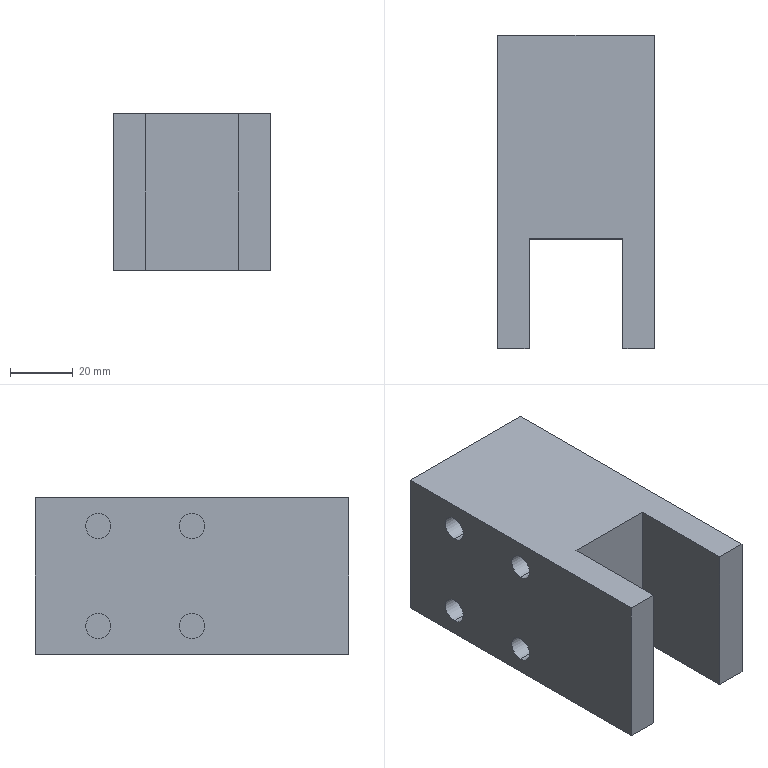Part | SolidWorks | features ICE 4, Extrusion 1 | 1 solid | 37 faces | box 50 x 100 x 50 mm | volume 185436 mm3 | plane 19 | cylinder 18 | commonest cylinder face diameters 8 x16 32 x2
STEP:
#1=CARTESIAN_POINT('',(15.,80.,-20.));
#2=VERTEX_POINT('',#1);
#3=CARTESIAN_POINT('',(15.,80.,-12.));
#4=VERTEX_POINT('',#3);
#5=CARTESIAN_POINT('',(15.,80.,-16.));
#6=DIRECTION('',(-1.,0.,0.));
#7=DIRECTION('',(0.,0.,-1.));
#8=AXIS2_PLACEMENT_3D('',#5,#6,#7);
#9=CIRCLE('',#8,4.);
#10=EDGE_CURVE('',#2,#4,#9,.T.);
#11=ORIENTED_EDGE('',*,*,#10,.T.);
#12=CARTESIAN_POINT('',(25.,80.,-12.));
#13=VERTEX_POINT('',#12);
#14=CARTESIAN_POINT('',(15.,80.,-12.));
#15=DIRECTION('',(1.,0.,0.));
#16=VECTOR('',#15,1000.);
#17=LINE('',#14,#16);
#18=EDGE_CURVE('',#4,#13,#17,.T.);
#19=ORIENTED_EDGE('',*,*,#18,.T.);
#20=CARTESIAN_POINT('',(25.,80.,-20.));
#21=VERTEX_POINT('',#20);
#22=CARTESIAN_POINT('',(25.,80.,-16.));
#23=DIRECTION('',(-1.,0.,0.));
#24=DIRECTION('',(0.,0.,-1.));
#25=AXIS2_PLACEMENT_3D('',#22,#23,#24);
#26=CIRCLE('',#25,4.);
#27=EDGE_CURVE('',#21,#13,#26,.T.);
#28=ORIENTED_EDGE('',*,*,#27,.F.);
#29=CARTESIAN_POINT('',(15.,80.,-20.));
#30=DIRECTION('',(1.,0.,0.));
#31=VECTOR('',#30,1000.);
#32=LINE('',#29,#31);
#33=EDGE_CURVE('',#2,#21,#32,.T.);
#34=ORIENTED_EDGE('',*,*,#33,.F.);
#35=EDGE_LOOP('',(#11,#19,#28,#34));
#36=FACE_OUTER_BOUND('',#35,.T.);
#37=CARTESIAN_POINT('',(15.,80.,-16.));
#38=DIRECTION('',(1.,0.,0.));
#39=DIRECTION('',(0.,0.,-1.));
#40=AXIS2_PLACEMENT_3D('',#37,#38,#39);
#41=CYLINDRICAL_SURFACE('',#40,4.);
#42=ADVANCED_FACE('',(#36),#41,.F.);
#43=CARTESIAN_POINT('',(15.,50.,-20.));
#44=VERTEX_POINT('',#43);
#45=CARTESIAN_POINT('',(15.,50.,-12.));
#46=VERTEX_POINT('',#45);
#47=CARTESIAN_POINT('',(15.,50.,-16.));
#48=DIRECTION('',(-1.,0.,0.));
#49=DIRECTION('',(0.,0.,-1.));
#50=AXIS2_PLACEMENT_3D('',#47,#48,#49);
#51=CIRCLE('',#50,4.);
#52=EDGE_CURVE('',#44,#46,#51,.T.);
#53=ORIENTED_EDGE('',*,*,#52,.T.);
#54=CARTESIAN_POINT('',(25.,50.,-12.));
#55=VERTEX_POINT('',#54);
#56=CARTESIAN_POINT('',(15.,50.,-12.));
#57=DIRECTION('',(1.,0.,0.));
#58=VECTOR('',#57,1000.);
#59=LINE('',#56,#58);
#60=EDGE_CURVE('',#46,#55,#59,.T.);
#61=ORIENTED_EDGE('',*,*,#60,.T.);
#62=CARTESIAN_POINT('',(25.,50.,-20.));
#63=VERTEX_POINT('',#62);
#64=CARTESIAN_POINT('',(25.,50.,-16.));
#65=DIRECTION('',(-1.,0.,0.));
#66=DIRECTION('',(0.,0.,-1.));
#67=AXIS2_PLACEMENT_3D('',#64,#65,#66);
#68=CIRCLE('',#67,4.);
#69=EDGE_CURVE('',#63,#55,#68,.T.);
#70=ORIENTED_EDGE('',*,*,#69,.F.);
#71=CARTESIAN_POINT('',(15.,50.,-20.));
#72=DIRECTION('',(1.,0.,0.));
#73=VECTOR('',#72,1000.);
#74=LINE('',#71,#73);
#75=EDGE_CURVE('',#44,#63,#74,.T.);
#76=ORIENTED_EDGE('',*,*,#75,.F.);
#77=EDGE_LOOP('',(#53,#61,#70,#76));
#78=FACE_OUTER_BOUND('',#77,.T.);
#79=CARTESIAN_POINT('',(15.,50.,-16.));
#80=DIRECTION('',(1.,0.,0.));
#81=DIRECTION('',(0.,0.,-1.));
#82=AXIS2_PLACEMENT_3D('',#79,#80,#81);
#83=CYLINDRICAL_SURFACE('',#82,4.);
#84=ADVANCED_FACE('',(#78),#83,.F.);
#85=CARTESIAN_POINT('',(15.,50.,20.));
#86=VERTEX_POINT('',#85);
#87=CARTESIAN_POINT('',(15.,50.,12.));
#88=VERTEX_POINT('',#87);
#89=CARTESIAN_POINT('',(15.,50.,16.));
#90=DIRECTION('',(1.,0.,0.));
#91=DIRECTION('',(0.,0.,-1.));
#92=AXIS2_PLACEMENT_3D('',#89,#90,#91);
#93=CIRCLE('',#92,4.);
#94=EDGE_CURVE('',#86,#88,#93,.T.);
#95=ORIENTED_EDGE('',*,*,#94,.F.);
#96=CARTESIAN_POINT('',(25.,50.,20.));
#97=VERTEX_POINT('',#96);
#98=CARTESIAN_POINT('',(15.,50.,20.));
#99=DIRECTION('',(1.,0.,0.));
#100=VECTOR('',#99,1000.);
#101=LINE('',#98,#100);
#102=EDGE_CURVE('',#86,#97,#101,.T.);
#103=ORIENTED_EDGE('',*,*,#102,.T.);
#104=CARTESIAN_POINT('',(25.,50.,12.));
#105=VERTEX_POINT('',#104);
#106=CARTESIAN_POINT('',(25.,50.,16.));
#107=DIRECTION('',(1.,0.,0.));
#108=DIRECTION('',(0.,0.,-1.));
#109=AXIS2_PLACEMENT_3D('',#106,#107,#108);
#110=CIRCLE('',#109,4.);
#111=EDGE_CURVE('',#97,#105,#110,.T.);
#112=ORIENTED_EDGE('',*,*,#111,.T.);
#113=CARTESIAN_POINT('',(15.,50.,12.));
#114=DIRECTION('',(1.,0.,0.));
#115=VECTOR('',#114,1000.);
#116=LINE('',#113,#115);
#117=EDGE_CURVE('',#88,#105,#116,.T.);
#118=ORIENTED_EDGE('',*,*,#117,.F.);
#119=EDGE_LOOP('',(#95,#103,#112,#118));
#120=FACE_OUTER_BOUND('',#119,.T.);
#121=CARTESIAN_POINT('',(15.,50.,16.));
#122=DIRECTION('',(1.,0.,0.));
#123=DIRECTION('',(0.,0.,-1.));
#124=AXIS2_PLACEMENT_3D('',#121,#122,#123);
#125=CYLINDRICAL_SURFACE('',#124,4.);
#126=ADVANCED_FACE('',(#120),#125,.F.);
#127=CARTESIAN_POINT('',(15.,80.,20.));
#128=VERTEX_POINT('',#127);
#129=CARTESIAN_POINT('',(15.,80.,12.));
#130=VERTEX_POINT('',#129);
#131=CARTESIAN_POINT('',(15.,80.,16.));
#132=DIRECTION('',(1.,0.,0.));
#133=DIRECTION('',(0.,0.,-1.));
#134=AXIS2_PLACEMENT_3D('',#131,#132,#133);
#135=CIRCLE('',#134,4.);
#136=EDGE_CURVE('',#128,#130,#135,.T.);
#137=ORIENTED_EDGE('',*,*,#136,.F.);
#138=CARTESIAN_POINT('',(25.,80.,20.));
#139=VERTEX_POINT('',#138);
#140=CARTESIAN_POINT('',(15.,80.,20.));
#141=DIRECTION('',(1.,0.,0.));
#142=VECTOR('',#141,1000.);
#143=LINE('',#140,#142);
#144=EDGE_CURVE('',#128,#139,#143,.T.);
#145=ORIENTED_EDGE('',*,*,#144,.T.);
#146=CARTESIAN_POINT('',(25.,80.,12.));
#147=VERTEX_POINT('',#146);
#148=CARTESIAN_POINT('',(25.,80.,16.));
#149=DIRECTION('',(1.,0.,0.));
#150=DIRECTION('',(0.,0.,-1.));
#151=AXIS2_PLACEMENT_3D('',#148,#149,#150);
#152=CIRCLE('',#151,4.);
#153=EDGE_CURVE('',#139,#147,#152,.T.);
#154=ORIENTED_EDGE('',*,*,#153,.T.);
#155=CARTESIAN_POINT('',(15.,80.,12.));
#156=DIRECTION('',(1.,0.,0.));
#157=VECTOR('',#156,1000.);
#158=LINE('',#155,#157);
#159=EDGE_CURVE('',#130,#147,#158,.T.);
#160=ORIENTED_EDGE('',*,*,#159,.F.);
#161=EDGE_LOOP('',(#137,#145,#154,#160));
#162=FACE_OUTER_BOUND('',#161,.T.);
#163=CARTESIAN_POINT('',(15.,80.,16.));
#164=DIRECTION('',(1.,0.,0.));
#165=DIRECTION('',(0.,0.,-1.));
#166=AXIS2_PLACEMENT_3D('',#163,#164,#165);
#167=CYLINDRICAL_SURFACE('',#166,4.);
#168=ADVANCED_FACE('',(#162),#167,.F.);
#169=CARTESIAN_POINT('',(-15.,50.,-20.));
#170=VERTEX_POINT('',#169);
#171=CARTESIAN_POINT('',(-15.,50.,-12.));
#172=VERTEX_POINT('',#171);
#173=CARTESIAN_POINT('',(-15.,50.,-16.));
#174=DIRECTION('',(-1.,0.,0.));
#175=DIRECTION('',(0.,0.,1.));
#176=AXIS2_PLACEMENT_3D('',#173,#174,#175);
#177=CIRCLE('',#176,4.);
#178=EDGE_CURVE('',#170,#172,#177,.T.);
#179=ORIENTED_EDGE('',*,*,#178,.F.);
#180=CARTESIAN_POINT('',(-25.,50.,-20.));
#181=VERTEX_POINT('',#180);
#182=CARTESIAN_POINT('',(-15.,50.,-20.));
#183=DIRECTION('',(-1.,0.,0.));
#184=VECTOR('',#183,1000.);
#185=LINE('',#182,#184);
#186=EDGE_CURVE('',#170,#181,#185,.T.);
#187=ORIENTED_EDGE('',*,*,#186,.T.);
#188=CARTESIAN_POINT('',(-25.,50.,-12.));
#189=VERTEX_POINT('',#188);
#190=CARTESIAN_POINT('',(-25.,50.,-16.));
#191=DIRECTION('',(-1.,0.,0.));
#192=DIRECTION('',(0.,0.,1.));
#193=AXIS2_PLACEMENT_3D('',#190,#191,#192);
#194=CIRCLE('',#193,4.);
#195=EDGE_CURVE('',#181,#189,#194,.T.);
#196=ORIENTED_EDGE('',*,*,#195,.T.);
#197=CARTESIAN_POINT('',(-15.,50.,-12.));
#198=DIRECTION('',(-1.,0.,0.));
#199=VECTOR('',#198,1000.);
#200=LINE('',#197,#199);
#201=EDGE_CURVE('',#172,#189,#200,.T.);
#202=ORIENTED_EDGE('',*,*,#201,.F.);
#203=EDGE_LOOP('',(#179,#187,#196,#202));
#204=FACE_OUTER_BOUND('',#203,.T.);
#205=CARTESIAN_POINT('',(-15.,50.,-16.));
#206=DIRECTION('',(-1.,0.,0.));
#207=DIRECTION('',(0.,0.,1.));
#208=AXIS2_PLACEMENT_3D('',#205,#206,#207);
#209=CYLINDRICAL_SURFACE('',#208,4.);
#210=ADVANCED_FACE('',(#204),#209,.F.);
#211=CARTESIAN_POINT('',(-15.,50.,20.));
#212=VERTEX_POINT('',#211);
#213=CARTESIAN_POINT('',(-15.,50.,12.));
#214=VERTEX_POINT('',#213);
#215=CARTESIAN_POINT('',(-15.,50.,16.));
#216=DIRECTION('',(1.,0.,0.));
#217=DIRECTION('',(0.,0.,1.));
#218=AXIS2_PLACEMENT_3D('',#215,#216,#217);
#219=CIRCLE('',#218,4.);
#220=EDGE_CURVE('',#212,#214,#219,.T.);
#221=ORIENTED_EDGE('',*,*,#220,.T.);
#222=CARTESIAN_POINT('',(-25.,50.,12.));
#223=VERTEX_POINT('',#222);
#224=CARTESIAN_POINT('',(-15.,50.,12.));
#225=DIRECTION('',(-1.,0.,0.));
#226=VECTOR('',#225,1000.);
#227=LINE('',#224,#226);
#228=EDGE_CURVE('',#214,#223,#227,.T.);
#229=ORIENTED_EDGE('',*,*,#228,.T.);
#230=CARTESIAN_POINT('',(-25.,50.,20.));
#231=VERTEX_POINT('',#230);
#232=CARTESIAN_POINT('',(-25.,50.,16.));
#233=DIRECTION('',(1.,0.,0.));
#234=DIRECTION('',(0.,0.,1.));
#235=AXIS2_PLACEMENT_3D('',#232,#233,#234);
#236=CIRCLE('',#235,4.);
#237=EDGE_CURVE('',#231,#223,#236,.T.);
#238=ORIENTED_EDGE('',*,*,#237,.F.);
#239=CARTESIAN_POINT('',(-15.,50.,20.));
#240=DIRECTION('',(-1.,0.,0.));
#241=VECTOR('',#240,1000.);
#242=LINE('',#239,#241);
#243=EDGE_CURVE('',#212,#231,#242,.T.);
#244=ORIENTED_EDGE('',*,*,#243,.F.);
#245=EDGE_LOOP('',(#221,#229,#238,#244));
#246=FACE_OUTER_BOUND('',#245,.T.);
#247=CARTESIAN_POINT('',(-15.,50.,16.));
#248=DIRECTION('',(-1.,0.,0.));
#249=DIRECTION('',(0.,0.,1.));
#250=AXIS2_PLACEMENT_3D('',#247,#248,#249);
#251=CYLINDRICAL_SURFACE('',#250,4.);
#252=ADVANCED_FACE('',(#246),#251,.F.);
#253=CARTESIAN_POINT('',(-15.,80.,20.));
#254=VERTEX_POINT('',#253);
#255=CARTESIAN_POINT('',(-15.,80.,12.));
#256=VERTEX_POINT('',#255);
#257=CARTESIAN_POINT('',(-15.,80.,16.));
#258=DIRECTION('',(1.,0.,0.));
#259=DIRECTION('',(0.,0.,1.));
#260=AXIS2_PLACEMENT_3D('',#257,#258,#259);
#261=CIRCLE('',#260,4.);
#262=EDGE_CURVE('',#254,#256,#261,.T.);
#263=ORIENTED_EDGE('',*,*,#262,.T.);
#264=CARTESIAN_POINT('',(-25.,80.,12.));
#265=VERTEX_POINT('',#264);
#266=CARTESIAN_POINT('',(-15.,80.,12.));
#267=DIRECTION('',(-1.,0.,0.));
#268=VECTOR('',#267,1000.);
#269=LINE('',#266,#268);
#270=EDGE_CURVE('',#256,#265,#269,.T.);
#271=ORIENTED_EDGE('',*,*,#270,.T.);
#272=CARTESIAN_POINT('',(-25.,80.,20.));
#273=VERTEX_POINT('',#272);
#274=CARTESIAN_POINT('',(-25.,80.,16.));
#275=DIRECTION('',(1.,0.,0.));
#276=DIRECTION('',(0.,0.,1.));
#277=AXIS2_PLACEMENT_3D('',#274,#275,#276);
#278=CIRCLE('',#277,4.);
#279=EDGE_CURVE('',#273,#265,#278,.T.);
#280=ORIENTED_EDGE('',*,*,#279,.F.);
#281=CARTESIAN_POINT('',(-15.,80.,20.));
#282=DIRECTION('',(-1.,0.,0.));
#283=VECTOR('',#282,1000.);
#284=LINE('',#281,#283);
#285=EDGE_CURVE('',#254,#273,#284,.T.);
#286=ORIENTED_EDGE('',*,*,#285,.F.);
#287=EDGE_LOOP('',(#263,#271,#280,#286));
#288=FACE_OUTER_BOUND('',#287,.T.);
#289=CARTESIAN_POINT('',(-15.,80.,16.));
#290=DIRECTION('',(-1.,0.,0.));
#291=DIRECTION('',(0.,0.,1.));
#292=AXIS2_PLACEMENT_3D('',#289,#290,#291);
#293=CYLINDRICAL_SURFACE('',#292,4.);
#294=ADVANCED_FACE('',(#288),#293,.F.);
#295=CARTESIAN_POINT('',(-15.,80.,-20.));
#296=VERTEX_POINT('',#295);
#297=CARTESIAN_POINT('',(-15.,80.,-12.));
#298=VERTEX_POINT('',#297);
#299=CARTESIAN_POINT('',(-15.,80.,-16.));
#300=DIRECTION('',(-1.,0.,0.));
#301=DIRECTION('',(0.,0.,1.));
#302=AXIS2_PLACEMENT_3D('',#299,#300,#301);
#303=CIRCLE('',#302,4.);
#304=EDGE_CURVE('',#296,#298,#303,.T.);
#305=ORIENTED_EDGE('',*,*,#304,.F.);
#306=CARTESIAN_POINT('',(-25.,80.,-20.));
#307=VERTEX_POINT('',#306);
#308=CARTESIAN_POINT('',(-15.,80.,-20.));
#309=DIRECTION('',(-1.,0.,0.));
#310=VECTOR('',#309,1000.);
#311=LINE('',#308,#310);
#312=EDGE_CURVE('',#296,#307,#311,.T.);
#313=ORIENTED_EDGE('',*,*,#312,.T.);
#314=CARTESIAN_POINT('',(-25.,80.,-12.));
#315=VERTEX_POINT('',#314);
#316=CARTESIAN_POINT('',(-25.,80.,-16.));
#317=DIRECTION('',(-1.,0.,0.));
#318=DIRECTION('',(0.,0.,1.));
#319=AXIS2_PLACEMENT_3D('',#316,#317,#318);
#320=CIRCLE('',#319,4.);
#321=EDGE_CURVE('',#307,#315,#320,.T.);
#322=ORIENTED_EDGE('',*,*,#321,.T.);
#323=CARTESIAN_POINT('',(-15.,80.,-12.));
#324=DIRECTION('',(-1.,0.,0.));
#325=VECTOR('',#324,1000.);
#326=LINE('',#323,#325);
#327=EDGE_CURVE('',#298,#315,#326,.T.);
#328=ORIENTED_EDGE('',*,*,#327,.F.);
#329=EDGE_LOOP('',(#305,#313,#322,#328));
#330=FACE_OUTER_BOUND('',#329,.T.);
#331=CARTESIAN_POINT('',(-15.,80.,-16.));
#332=DIRECTION('',(-1.,0.,0.));
#333=DIRECTION('',(0.,0.,1.));
#334=AXIS2_PLACEMENT_3D('',#331,#332,#333);
#335=CYLINDRICAL_SURFACE('',#334,4.);
#336=ADVANCED_FACE('',(#330),#335,.F.);
#337=CARTESIAN_POINT('',(0.,90.,-16.));
#338=VERTEX_POINT('',#337);
#339=CARTESIAN_POINT('',(0.,90.,16.));
#340=VERTEX_POINT('',#339);
#341=CARTESIAN_POINT('',(0.,90.,0.));
#342=DIRECTION('',(0.,1.,0.));
#343=DIRECTION('',(0.,0.,1.));
#344=AXIS2_PLACEMENT_3D('',#341,#342,#343);
#345=CIRCLE('',#344,16.);
#346=EDGE_CURVE('',#338,#340,#345,.T.);
#347=ORIENTED_EDGE('',*,*,#346,.F.);
#348=CARTESIAN_POINT('',(0.,100.,-16.));
#349=VERTEX_POINT('',#348);
#350=CARTESIAN_POINT('',(0.,90.,-16.));
#351=DIRECTION('',(0.,1.,0.));
#352=VECTOR('',#351,1000.);
#353=LINE('',#350,#352);
#354=EDGE_CURVE('',#338,#349,#353,.T.);
#355=ORIENTED_EDGE('',*,*,#354,.T.);
#356=CARTESIAN_POINT('',(0.,100.,16.));
#357=VERTEX_POINT('',#356);
#358=CARTESIAN_POINT('',(0.,100.,0.));
#359=DIRECTION('',(0.,1.,0.));
#360=DIRECTION('',(0.,0.,1.));
#361=AXIS2_PLACEMENT_3D('',#358,#359,#360);
#362=CIRCLE('',#361,16.);
#363=EDGE_CURVE('',#349,#357,#362,.T.);
#364=ORIENTED_EDGE('',*,*,#363,.T.);
#365=CARTESIAN_POINT('',(0.,90.,16.));
#366=DIRECTION('',(0.,1.,0.));
#367=VECTOR('',#366,1000.);
#368=LINE('',#365,#367);
#369=EDGE_CURVE('',#340,#357,#368,.T.);
#370=ORIENTED_EDGE('',*,*,#369,.F.);
#371=EDGE_LOOP('',(#347,#355,#364,#370));
#372=FACE_OUTER_BOUND('',#371,.T.);
#373=CARTESIAN_POINT('',(0.,90.,0.));
#374=DIRECTION('',(0.,1.,0.));
#375=DIRECTION('',(0.,0.,1.));
#376=AXIS2_PLACEMENT_3D('',#373,#374,#375);
#377=CYLINDRICAL_SURFACE('',#376,16.);
#378=ADVANCED_FACE('',(#372),#377,.F.);
#379=CARTESIAN_POINT('',(25.,50.,16.));
#380=DIRECTION('',(1.,0.,0.));
#381=DIRECTION('',(0.,0.,-1.));
#382=AXIS2_PLACEMENT_3D('',#379,#380,#381);
#383=CIRCLE('',#382,4.);
#384=EDGE_CURVE('',#105,#97,#383,.T.);
#385=ORIENTED_EDGE('',*,*,#384,.F.);
#386=ORIENTED_EDGE('',*,*,#111,.F.);
#387=EDGE_LOOP('',(#385,#386));
#388=FACE_BOUND('',#387,.T.);
#389=CARTESIAN_POINT('',(25.,80.,16.));
#390=DIRECTION('',(1.,0.,0.));
#391=DIRECTION('',(0.,0.,-1.));
#392=AXIS2_PLACEMENT_3D('',#389,#390,#391);
#393=CIRCLE('',#392,4.);
#394=EDGE_CURVE('',#147,#139,#393,.T.);
#395=ORIENTED_EDGE('',*,*,#394,.F.);
#396=ORIENTED_EDGE('',*,*,#153,.F.);
#397=EDGE_LOOP('',(#395,#396));
#398=FACE_BOUND('',#397,.T.);
#399=CARTESIAN_POINT('',(25.,0.,25.));
#400=VERTEX_POINT('',#399);
#401=CARTESIAN_POINT('',(25.,0.,-25.));
#402=VERTEX_POINT('',#401);
#403=CARTESIAN_POINT('',(25.,0.,-25.));
#404=DIRECTION('',(0.,0.,-1.));
#405=VECTOR('',#404,1000.);
#406=LINE('',#403,#405);
#407=EDGE_CURVE('',#400,#402,#406,.T.);
#408=ORIENTED_EDGE('',*,*,#407,.T.);
#409=CARTESIAN_POINT('',(25.,100.,-25.));
#410=VERTEX_POINT('',#409);
#411=CARTESIAN_POINT('',(25.,100.,-25.));
#412=DIRECTION('',(0.,-1.,0.));
#413=VECTOR('',#412,1000.);
#414=LINE('',#411,#413);
#415=EDGE_CURVE('',#410,#402,#414,.T.);
#416=ORIENTED_EDGE('',*,*,#415,.F.);
#417=CARTESIAN_POINT('',(25.,100.,25.));
#418=VERTEX_POINT('',#417);
#419=CARTESIAN_POINT('',(25.,100.,-25.));
#420=DIRECTION('',(0.,0.,-1.));
#421=VECTOR('',#420,1000.);
#422=LINE('',#419,#421);
#423=EDGE_CURVE('',#418,#410,#422,.T.);
#424=ORIENTED_EDGE('',*,*,#423,.F.);
#425=CARTESIAN_POINT('',(25.,100.,25.));
#426=DIRECTION('',(0.,-1.,0.));
#427=VECTOR('',#426,1000.);
#428=LINE('',#425,#427);
#429=EDGE_CURVE('',#418,#400,#428,.T.);
#430=ORIENTED_EDGE('',*,*,#429,.T.);
#431=EDGE_LOOP('',(#408,#416,#424,#430));
#432=FACE_OUTER_BOUND('',#431,.T.);
#433=ORIENTED_EDGE('',*,*,#69,.T.);
#434=CARTESIAN_POINT('',(25.,50.,-16.));
#435=DIRECTION('',(-1.,0.,0.));
#436=DIRECTION('',(0.,0.,-1.));
#437=AXIS2_PLACEMENT_3D('',#434,#435,#436);
#438=CIRCLE('',#437,4.);
#439=EDGE_CURVE('',#55,#63,#438,.T.);
#440=ORIENTED_EDGE('',*,*,#439,.T.);
#441=EDGE_LOOP('',(#433,#440));
#442=FACE_BOUND('',#441,.T.);
#443=ORIENTED_EDGE('',*,*,#27,.T.);
#444=CARTESIAN_POINT('',(25.,80.,-16.));
#445=DIRECTION('',(-1.,0.,0.));
#446=DIRECTION('',(0.,0.,-1.));
#447=AXIS2_PLACEMENT_3D('',#444,#445,#446);
#448=CIRCLE('',#447,4.);
#449=EDGE_CURVE('',#13,#21,#448,.T.);
#450=ORIENTED_EDGE('',*,*,#449,.T.);
#451=EDGE_LOOP('',(#443,#450));
#452=FACE_BOUND('',#451,.T.);
#453=CARTESIAN_POINT('',(25.,100.,-25.));
#454=DIRECTION('',(-1.,0.,0.));
#455=DIRECTION('',(0.,0.,1.));
#456=AXIS2_PLACEMENT_3D('',#453,#454,#455);
#457=PLANE('',#456);
#458=ADVANCED_FACE('',(#388,#398,#432,#442,#452),#457,.F.);
#459=CARTESIAN_POINT('',(-25.,50.,-16.));
#460=DIRECTION('',(-1.,0.,0.));
#461=DIRECTION('',(0.,0.,1.));
#462=AXIS2_PLACEMENT_3D('',#459,#460,#461);
#463=CIRCLE('',#462,4.);
#464=EDGE_CURVE('',#189,#181,#463,.T.);
#465=ORIENTED_EDGE('',*,*,#464,.F.);
#466=ORIENTED_EDGE('',*,*,#195,.F.);
#467=EDGE_LOOP('',(#465,#466));
#468=FACE_BOUND('',#467,.T.);
#469=CARTESIAN_POINT('',(-25.,80.,-16.));
#470=DIRECTION('',(-1.,0.,0.));
#471=DIRECTION('',(0.,0.,1.));
#472=AXIS2_PLACEMENT_3D('',#469,#470,#471);
#473=CIRCLE('',#472,4.);
#474=EDGE_CURVE('',#315,#307,#473,.T.);
#475=ORIENTED_EDGE('',*,*,#474,.F.);
#476=ORIENTED_EDGE('',*,*,#321,.F.);
#477=EDGE_LOOP('',(#475,#476));
#478=FACE_BOUND('',#477,.T.);
#479=CARTESIAN_POINT('',(-25.,0.,-25.));
#480=VERTEX_POINT('',#479);
#481=CARTESIAN_POINT('',(-25.,0.,25.));
#482=VERTEX_POINT('',#481);
#483=CARTESIAN_POINT('',(-25.,0.,-25.));
#484=DIRECTION('',(0.,0.,1.));
#485=VECTOR('',#484,1000.);
#486=LINE('',#483,#485);
#487=EDGE_CURVE('',#480,#482,#486,.T.);
#488=ORIENTED_EDGE('',*,*,#487,.T.);
#489=CARTESIAN_POINT('',(-25.,100.,25.));
#490=VERTEX_POINT('',#489);
#491=CARTESIAN_POINT('',(-25.,100.,25.));
#492=DIRECTION('',(0.,-1.,0.));
#493=VECTOR('',#492,1000.);
#494=LINE('',#491,#493);
#495=EDGE_CURVE('',#490,#482,#494,.T.);
#496=ORIENTED_EDGE('',*,*,#495,.F.);
#497=CARTESIAN_POINT('',(-25.,100.,-25.));
#498=VERTEX_POINT('',#497);
#499=CARTESIAN_POINT('',(-25.,100.,-25.));
#500=DIRECTION('',(0.,0.,1.));
#501=VECTOR('',#500,1000.);
#502=LINE('',#499,#501);
#503=EDGE_CURVE('',#498,#490,#502,.T.);
#504=ORIENTED_EDGE('',*,*,#503,.F.);
#505=CARTESIAN_POINT('',(-25.,100.,-25.));
#506=DIRECTION('',(0.,-1.,0.));
#507=VECTOR('',#506,1000.);
#508=LINE('',#505,#507);
#509=EDGE_CURVE('',#498,#480,#508,.T.);
#510=ORIENTED_EDGE('',*,*,#509,.T.);
#511=EDGE_LOOP('',(#488,#496,#504,#510));
#512=FACE_OUTER_BOUND('',#511,.T.);
#513=ORIENTED_EDGE('',*,*,#279,.T.);
#514=CARTESIAN_POINT('',(-25.,80.,16.));
#515=DIRECTION('',(1.,0.,0.));
#516=DIRECTION('',(0.,0.,1.));
#517=AXIS2_PLACEMENT_3D('',#514,#515,#516);
#518=CIRCLE('',#517,4.);
#519=EDGE_CURVE('',#265,#273,#518,.T.);
#520=ORIENTED_EDGE('',*,*,#519,.T.);
#521=EDGE_LOOP('',(#513,#520));
#522=FACE_BOUND('',#521,.T.);
#523=ORIENTED_EDGE('',*,*,#237,.T.);
#524=CARTESIAN_POINT('',(-25.,50.,16.));
#525=DIRECTION('',(1.,0.,0.));
#526=DIRECTION('',(0.,0.,1.));
#527=AXIS2_PLACEMENT_3D('',#524,#525,#526);
#528=CIRCLE('',#527,4.);
#529=EDGE_CURVE('',#223,#231,#528,.T.);
#530=ORIENTED_EDGE('',*,*,#529,.T.);
#531=EDGE_LOOP('',(#523,#530));
#532=FACE_BOUND('',#531,.T.);
#533=CARTESIAN_POINT('',(-25.,100.,-25.));
#534=DIRECTION('',(1.,0.,0.));
#535=DIRECTION('',(0.,0.,-1.));
#536=AXIS2_PLACEMENT_3D('',#533,#534,#535);
#537=PLANE('',#536);
#538=ADVANCED_FACE('',(#468,#478,#512,#522,#532),#537,.F.);
#539=CARTESIAN_POINT('',(15.,0.,25.));
#540=VERTEX_POINT('',#539);
#541=CARTESIAN_POINT('',(-25.,0.,25.));
#542=DIRECTION('',(1.,0.,0.));
#543=VECTOR('',#542,1000.);
#544=LINE('',#541,#543);
#545=EDGE_CURVE('',#540,#400,#544,.T.);
#546=ORIENTED_EDGE('',*,*,#545,.F.);
#547=CARTESIAN_POINT('',(15.,0.,-25.));
#548=VERTEX_POINT('',#547);
#549=CARTESIAN_POINT('',(15.,0.,25.));
#550=DIRECTION('',(0.,0.,1.));
#551=VECTOR('',#550,1000.);
#552=LINE('',#549,#551);
#553=EDGE_CURVE('',#548,#540,#552,.T.);
#554=ORIENTED_EDGE('',*,*,#553,.F.);
#555=CARTESIAN_POINT('',(-25.,0.,-25.));
#556=DIRECTION('',(-1.,0.,0.));
#557=VECTOR('',#556,1000.);
#558=LINE('',#555,#557);
#559=EDGE_CURVE('',#402,#548,#558,.T.);
#560=ORIENTED_EDGE('',*,*,#559,.F.);
#561=ORIENTED_EDGE('',*,*,#407,.F.);
#562=EDGE_LOOP('',(#546,#554,#560,#561));
#563=FACE_OUTER_BOUND('',#562,.T.);
#564=CARTESIAN_POINT('',(0.,0.,0.));
#565=DIRECTION('',(0.,1.,0.));
#566=DIRECTION('',(0.,0.,1.));
#567=AXIS2_PLACEMENT_3D('',#564,#565,#566);
#568=PLANE('',#567);
#569=ADVANCED_FACE('',(#563),#568,.F.);
#570=ORIENTED_EDGE('',*,*,#559,.T.);
#571=CARTESIAN_POINT('',(15.,35.,-25.));
#572=VERTEX_POINT('',#571);
#573=CARTESIAN_POINT('',(15.,35.,-25.));
#574=DIRECTION('',(0.,-1.,0.));
#575=VECTOR('',#574,1000.);
#576=LINE('',#573,#575);
#577=EDGE_CURVE('',#572,#548,#576,.T.);
#578=ORIENTED_EDGE('',*,*,#577,.F.);
#579=CARTESIAN_POINT('',(-15.,35.,-25.));
#580=VERTEX_POINT('',#579);
#581=CARTESIAN_POINT('',(-15.,35.,-25.));
#582=DIRECTION('',(1.,0.,0.));
#583=VECTOR('',#582,1000.);
#584=LINE('',#581,#583);
#585=EDGE_CURVE('',#580,#572,#584,.T.);
#586=ORIENTED_EDGE('',*,*,#585,.F.);
#587=CARTESIAN_POINT('',(-15.,0.,-25.));
#588=VERTEX_POINT('',#587);
#589=CARTESIAN_POINT('',(-15.,35.,-25.));
#590=DIRECTION('',(0.,-1.,0.));
#591=VECTOR('',#590,1000.);
#592=LINE('',#589,#591);
#593=EDGE_CURVE('',#580,#588,#592,.T.);
#594=ORIENTED_EDGE('',*,*,#593,.T.);
#595=CARTESIAN_POINT('',(-25.,0.,-25.));
#596=DIRECTION('',(-1.,0.,0.));
#597=VECTOR('',#596,1000.);
#598=LINE('',#595,#597);
#599=EDGE_CURVE('',#588,#480,#598,.T.);
#600=ORIENTED_EDGE('',*,*,#599,.T.);
#601=ORIENTED_EDGE('',*,*,#509,.F.);
#602=CARTESIAN_POINT('',(-25.,100.,-25.));
#603=DIRECTION('',(-1.,0.,0.));
#604=VECTOR('',#603,1000.);
#605=LINE('',#602,#604);
#606=EDGE_CURVE('',#410,#498,#605,.T.);
#607=ORIENTED_EDGE('',*,*,#606,.F.);
#608=ORIENTED_EDGE('',*,*,#415,.T.);
#609=EDGE_LOOP('',(#570,#578,#586,#594,#600,#601,#607,#608));
#610=FACE_OUTER_BOUND('',#609,.T.);
#611=CARTESIAN_POINT('',(-25.,100.,-25.));
#612=DIRECTION('',(0.,0.,1.));
#613=DIRECTION('',(1.,0.,0.));
#614=AXIS2_PLACEMENT_3D('',#611,#612,#613);
#615=PLANE('',#614);
#616=ADVANCED_FACE('',(#610),#615,.F.);
#617=CARTESIAN_POINT('',(15.,35.,25.));
#618=VERTEX_POINT('',#617);
#619=CARTESIAN_POINT('',(-15.,35.,25.));
#620=VERTEX_POINT('',#619);
#621=CARTESIAN_POINT('',(-15.,35.,25.));
#622=DIRECTION('',(-1.,0.,0.));
#623=VECTOR('',#622,1000.);
#624=LINE('',#621,#623);
#625=EDGE_CURVE('',#618,#620,#624,.T.);
#626=ORIENTED_EDGE('',*,*,#625,.F.);
#627=CARTESIAN_POINT('',(15.,35.,25.));
#628=DIRECTION('',(0.,-1.,0.));
#629=VECTOR('',#628,1000.);
#630=LINE('',#627,#629);
#631=EDGE_CURVE('',#618,#540,#630,.T.);
#632=ORIENTED_EDGE('',*,*,#631,.T.);
#633=ORIENTED_EDGE('',*,*,#545,.T.);
#634=ORIENTED_EDGE('',*,*,#429,.F.);
#635=CARTESIAN_POINT('',(-25.,100.,25.));
#636=DIRECTION('',(1.,0.,0.));
#637=VECTOR('',#636,1000.);
#638=LINE('',#635,#637);
#639=EDGE_CURVE('',#490,#418,#638,.T.);
#640=ORIENTED_EDGE('',*,*,#639,.F.);
#641=ORIENTED_EDGE('',*,*,#495,.T.);
#642=CARTESIAN_POINT('',(-15.,0.,25.));
#643=VERTEX_POINT('',#642);
#644=CARTESIAN_POINT('',(-25.,0.,25.));
#645=DIRECTION('',(1.,0.,0.));
#646=VECTOR('',#645,1000.);
#647=LINE('',#644,#646);
#648=EDGE_CURVE('',#482,#643,#647,.T.);
#649=ORIENTED_EDGE('',*,*,#648,.T.);
#650=CARTESIAN_POINT('',(-15.,35.,25.));
#651=DIRECTION('',(0.,-1.,0.));
#652=VECTOR('',#651,1000.);
#653=LINE('',#650,#652);
#654=EDGE_CURVE('',#620,#643,#653,.T.);
#655=ORIENTED_EDGE('',*,*,#654,.F.);
#656=EDGE_LOOP('',(#626,#632,#633,#634,#640,#641,#649,#655));
#657=FACE_OUTER_BOUND('',#656,.T.);
#658=CARTESIAN_POINT('',(-25.,100.,25.));
#659=DIRECTION('',(0.,0.,-1.));
#660=DIRECTION('',(-1.,0.,0.));
#661=AXIS2_PLACEMENT_3D('',#658,#659,#660);
#662=PLANE('',#661);
#663=ADVANCED_FACE('',(#657),#662,.F.);
#664=CARTESIAN_POINT('',(0.,100.,0.));
#665=DIRECTION('',(0.,1.,0.));
#666=DIRECTION('',(0.,0.,1.));
#667=AXIS2_PLACEMENT_3D('',#664,#665,#666);
#668=CIRCLE('',#667,16.);
#669=EDGE_CURVE('',#357,#349,#668,.T.);
#670=ORIENTED_EDGE('',*,*,#669,.F.);
#671=ORIENTED_EDGE('',*,*,#363,.F.);
#672=EDGE_LOOP('',(#670,#671));
#673=FACE_BOUND('',#672,.T.);
#674=ORIENTED_EDGE('',*,*,#423,.T.);
#675=ORIENTED_EDGE('',*,*,#606,.T.);
#676=ORIENTED_EDGE('',*,*,#503,.T.);
#677=ORIENTED_EDGE('',*,*,#639,.T.);
#678=EDGE_LOOP('',(#674,#675,#676,#677));
#679=FACE_OUTER_BOUND('',#678,.T.);
#680=CARTESIAN_POINT('',(0.,100.,0.));
#681=DIRECTION('',(0.,1.,0.));
#682=DIRECTION('',(0.,0.,1.));
#683=AXIS2_PLACEMENT_3D('',#680,#681,#682);
#684=PLANE('',#683);
#685=ADVANCED_FACE('',(#673,#679),#684,.T.);
#686=ORIENTED_EDGE('',*,*,#599,.F.);
#687=CARTESIAN_POINT('',(-15.,0.,25.));
#688=DIRECTION('',(0.,0.,-1.));
#689=VECTOR('',#688,1000.);
#690=LINE('',#687,#689);
#691=EDGE_CURVE('',#643,#588,#690,.T.);
#692=ORIENTED_EDGE('',*,*,#691,.F.);
#693=ORIENTED_EDGE('',*,*,#648,.F.);
#694=ORIENTED_EDGE('',*,*,#487,.F.);
#695=EDGE_LOOP('',(#686,#692,#693,#694));
#696=FACE_OUTER_BOUND('',#695,.T.);
#697=CARTESIAN_POINT('',(0.,0.,0.));
#698=DIRECTION('',(0.,1.,0.));
#699=DIRECTION('',(0.,0.,1.));
#700=AXIS2_PLACEMENT_3D('',#697,#698,#699);
#701=PLANE('',#700);
#702=ADVANCED_FACE('',(#696),#701,.F.);
#703=ORIENTED_EDGE('',*,*,#553,.T.);
#704=ORIENTED_EDGE('',*,*,#631,.F.);
#705=CARTESIAN_POINT('',(15.,35.,25.));
#706=DIRECTION('',(0.,0.,1.));
#707=VECTOR('',#706,1000.);
#708=LINE('',#705,#707);
#709=EDGE_CURVE('',#572,#618,#708,.T.);
#710=ORIENTED_EDGE('',*,*,#709,.F.);
#711=ORIENTED_EDGE('',*,*,#577,.T.);
#712=EDGE_LOOP('',(#703,#704,#710,#711));
#713=FACE_OUTER_BOUND('',#712,.T.);
#714=CARTESIAN_POINT('',(15.,35.,25.));
#715=DIRECTION('',(1.,0.,0.));
#716=DIRECTION('',(0.,0.,-1.));
#717=AXIS2_PLACEMENT_3D('',#714,#715,#716);
#718=PLANE('',#717);
#719=ADVANCED_FACE('',(#713),#718,.F.);
#720=ORIENTED_EDGE('',*,*,#691,.T.);
#721=ORIENTED_EDGE('',*,*,#593,.F.);
#722=CARTESIAN_POINT('',(-15.,35.,25.));
#723=DIRECTION('',(0.,0.,-1.));
#724=VECTOR('',#723,1000.);
#725=LINE('',#722,#724);
#726=EDGE_CURVE('',#620,#580,#725,.T.);
#727=ORIENTED_EDGE('',*,*,#726,.F.);
#728=ORIENTED_EDGE('',*,*,#654,.T.);
#729=EDGE_LOOP('',(#720,#721,#727,#728));
#730=FACE_OUTER_BOUND('',#729,.T.);
#731=CARTESIAN_POINT('',(-15.,35.,25.));
#732=DIRECTION('',(-1.,0.,0.));
#733=DIRECTION('',(0.,0.,1.));
#734=AXIS2_PLACEMENT_3D('',#731,#732,#733);
#735=PLANE('',#734);
#736=ADVANCED_FACE('',(#730),#735,.F.);
#737=ORIENTED_EDGE('',*,*,#709,.T.);
#738=ORIENTED_EDGE('',*,*,#625,.T.);
#739=ORIENTED_EDGE('',*,*,#726,.T.);
#740=ORIENTED_EDGE('',*,*,#585,.T.);
#741=EDGE_LOOP('',(#737,#738,#739,#740));
#742=FACE_OUTER_BOUND('',#741,.T.);
#743=CARTESIAN_POINT('',(0.,35.,0.));
#744=DIRECTION('',(0.,-1.,0.));
#745=DIRECTION('',(0.,0.,-1.));
#746=AXIS2_PLACEMENT_3D('',#743,#744,#745);
#747=PLANE('',#746);
#748=ADVANCED_FACE('',(#742),#747,.T.);
#749=ORIENTED_EDGE('',*,*,#354,.F.);
#750=CARTESIAN_POINT('',(0.,90.,0.));
#751=DIRECTION('',(0.,1.,0.));
#752=DIRECTION('',(0.,0.,1.));
#753=AXIS2_PLACEMENT_3D('',#750,#751,#752);
#754=CIRCLE('',#753,16.);
#755=EDGE_CURVE('',#340,#338,#754,.T.);
#756=ORIENTED_EDGE('',*,*,#755,.F.);
#757=ORIENTED_EDGE('',*,*,#369,.T.);
#758=ORIENTED_EDGE('',*,*,#669,.T.);
#759=EDGE_LOOP('',(#749,#756,#757,#758));
#760=FACE_OUTER_BOUND('',#759,.T.);
#761=CARTESIAN_POINT('',(0.,90.,0.));
#762=DIRECTION('',(0.,1.,0.));
#763=DIRECTION('',(0.,0.,1.));
#764=AXIS2_PLACEMENT_3D('',#761,#762,#763);
#765=CYLINDRICAL_SURFACE('',#764,16.);
#766=ADVANCED_FACE('',(#760),#765,.F.);
#767=ORIENTED_EDGE('',*,*,#755,.T.);
#768=ORIENTED_EDGE('',*,*,#346,.T.);
#769=EDGE_LOOP('',(#767,#768));
#770=FACE_OUTER_BOUND('',#769,.T.);
#771=CARTESIAN_POINT('',(0.,90.,0.));
#772=DIRECTION('',(0.,1.,0.));
#773=DIRECTION('',(0.,0.,1.));
#774=AXIS2_PLACEMENT_3D('',#771,#772,#773);
#775=PLANE('',#774);
#776=ADVANCED_FACE('',(#770),#775,.T.);
#777=ORIENTED_EDGE('',*,*,#312,.F.);
#778=CARTESIAN_POINT('',(-15.,80.,-16.));
#779=DIRECTION('',(-1.,0.,0.));
#780=DIRECTION('',(0.,0.,1.));
#781=AXIS2_PLACEMENT_3D('',#778,#779,#780);
#782=CIRCLE('',#781,4.);
#783=EDGE_CURVE('',#298,#296,#782,.T.);
#784=ORIENTED_EDGE('',*,*,#783,.F.);
#785=ORIENTED_EDGE('',*,*,#327,.T.);
#786=ORIENTED_EDGE('',*,*,#474,.T.);
#787=EDGE_LOOP('',(#777,#784,#785,#786));
#788=FACE_OUTER_BOUND('',#787,.T.);
#789=CARTESIAN_POINT('',(-15.,80.,-16.));
#790=DIRECTION('',(-1.,0.,0.));
#791=DIRECTION('',(0.,0.,1.));
#792=AXIS2_PLACEMENT_3D('',#789,#790,#791);
#793=CYLINDRICAL_SURFACE('',#792,4.);
#794=ADVANCED_FACE('',(#788),#793,.F.);
#795=ORIENTED_EDGE('',*,*,#783,.T.);
#796=ORIENTED_EDGE('',*,*,#304,.T.);
#797=EDGE_LOOP('',(#795,#796));
#798=FACE_OUTER_BOUND('',#797,.T.);
#799=CARTESIAN_POINT('',(-15.,0.,0.));
#800=DIRECTION('',(-1.,0.,0.));
#801=DIRECTION('',(0.,0.,1.));
#802=AXIS2_PLACEMENT_3D('',#799,#800,#801);
#803=PLANE('',#802);
#804=ADVANCED_FACE('',(#798),#803,.T.);
#805=ORIENTED_EDGE('',*,*,#270,.F.);
#806=CARTESIAN_POINT('',(-15.,80.,16.));
#807=DIRECTION('',(1.,0.,0.));
#808=DIRECTION('',(0.,0.,1.));
#809=AXIS2_PLACEMENT_3D('',#806,#807,#808);
#810=CIRCLE('',#809,4.);
#811=EDGE_CURVE('',#256,#254,#810,.T.);
#812=ORIENTED_EDGE('',*,*,#811,.T.);
#813=ORIENTED_EDGE('',*,*,#285,.T.);
#814=ORIENTED_EDGE('',*,*,#519,.F.);
#815=EDGE_LOOP('',(#805,#812,#813,#814));
#816=FACE_OUTER_BOUND('',#815,.T.);
#817=CARTESIAN_POINT('',(-15.,80.,16.));
#818=DIRECTION('',(-1.,0.,0.));
#819=DIRECTION('',(0.,0.,1.));
#820=AXIS2_PLACEMENT_3D('',#817,#818,#819);
#821=CYLINDRICAL_SURFACE('',#820,4.);
#822=ADVANCED_FACE('',(#816),#821,.F.);
#823=ORIENTED_EDGE('',*,*,#262,.F.);
#824=ORIENTED_EDGE('',*,*,#811,.F.);
#825=EDGE_LOOP('',(#823,#824));
#826=FACE_OUTER_BOUND('',#825,.T.);
#827=CARTESIAN_POINT('',(-15.,0.,0.));
#828=DIRECTION('',(-1.,0.,0.));
#829=DIRECTION('',(0.,0.,1.));
#830=AXIS2_PLACEMENT_3D('',#827,#828,#829);
#831=PLANE('',#830);
#832=ADVANCED_FACE('',(#826),#831,.T.);
#833=ORIENTED_EDGE('',*,*,#228,.F.);
#834=CARTESIAN_POINT('',(-15.,50.,16.));
#835=DIRECTION('',(1.,0.,0.));
#836=DIRECTION('',(0.,0.,1.));
#837=AXIS2_PLACEMENT_3D('',#834,#835,#836);
#838=CIRCLE('',#837,4.);
#839=EDGE_CURVE('',#214,#212,#838,.T.);
#840=ORIENTED_EDGE('',*,*,#839,.T.);
#841=ORIENTED_EDGE('',*,*,#243,.T.);
#842=ORIENTED_EDGE('',*,*,#529,.F.);
#843=EDGE_LOOP('',(#833,#840,#841,#842));
#844=FACE_OUTER_BOUND('',#843,.T.);
#845=CARTESIAN_POINT('',(-15.,50.,16.));
#846=DIRECTION('',(-1.,0.,0.));
#847=DIRECTION('',(0.,0.,1.));
#848=AXIS2_PLACEMENT_3D('',#845,#846,#847);
#849=CYLINDRICAL_SURFACE('',#848,4.);
#850=ADVANCED_FACE('',(#844),#849,.F.);
#851=ORIENTED_EDGE('',*,*,#220,.F.);
#852=ORIENTED_EDGE('',*,*,#839,.F.);
#853=EDGE_LOOP('',(#851,#852));
#854=FACE_OUTER_BOUND('',#853,.T.);
#855=CARTESIAN_POINT('',(-15.,0.,0.));
#856=DIRECTION('',(-1.,0.,0.));
#857=DIRECTION('',(0.,0.,1.));
#858=AXIS2_PLACEMENT_3D('',#855,#856,#857);
#859=PLANE('',#858);
#860=ADVANCED_FACE('',(#854),#859,.T.);
#861=ORIENTED_EDGE('',*,*,#186,.F.);
#862=CARTESIAN_POINT('',(-15.,50.,-16.));
#863=DIRECTION('',(-1.,0.,0.));
#864=DIRECTION('',(0.,0.,1.));
#865=AXIS2_PLACEMENT_3D('',#862,#863,#864);
#866=CIRCLE('',#865,4.);
#867=EDGE_CURVE('',#172,#170,#866,.T.);
#868=ORIENTED_EDGE('',*,*,#867,.F.);
#869=ORIENTED_EDGE('',*,*,#201,.T.);
#870=ORIENTED_EDGE('',*,*,#464,.T.);
#871=EDGE_LOOP('',(#861,#868,#869,#870));
#872=FACE_OUTER_BOUND('',#871,.T.);
#873=CARTESIAN_POINT('',(-15.,50.,-16.));
#874=DIRECTION('',(-1.,0.,0.));
#875=DIRECTION('',(0.,0.,1.));
#876=AXIS2_PLACEMENT_3D('',#873,#874,#875);
#877=CYLINDRICAL_SURFACE('',#876,4.);
#878=ADVANCED_FACE('',(#872),#877,.F.);
#879=ORIENTED_EDGE('',*,*,#867,.T.);
#880=ORIENTED_EDGE('',*,*,#178,.T.);
#881=EDGE_LOOP('',(#879,#880));
#882=FACE_OUTER_BOUND('',#881,.T.);
#883=CARTESIAN_POINT('',(-15.,0.,0.));
#884=DIRECTION('',(-1.,0.,0.));
#885=DIRECTION('',(0.,0.,1.));
#886=AXIS2_PLACEMENT_3D('',#883,#884,#885);
#887=PLANE('',#886);
#888=ADVANCED_FACE('',(#882),#887,.T.);
#889=ORIENTED_EDGE('',*,*,#144,.F.);
#890=CARTESIAN_POINT('',(15.,80.,16.));
#891=DIRECTION('',(1.,0.,0.));
#892=DIRECTION('',(0.,0.,-1.));
#893=AXIS2_PLACEMENT_3D('',#890,#891,#892);
#894=CIRCLE('',#893,4.);
#895=EDGE_CURVE('',#130,#128,#894,.T.);
#896=ORIENTED_EDGE('',*,*,#895,.F.);
#897=ORIENTED_EDGE('',*,*,#159,.T.);
#898=ORIENTED_EDGE('',*,*,#394,.T.);
#899=EDGE_LOOP('',(#889,#896,#897,#898));
#900=FACE_OUTER_BOUND('',#899,.T.);
#901=CARTESIAN_POINT('',(15.,80.,16.));
#902=DIRECTION('',(1.,0.,0.));
#903=DIRECTION('',(0.,0.,-1.));
#904=AXIS2_PLACEMENT_3D('',#901,#902,#903);
#905=CYLINDRICAL_SURFACE('',#904,4.);
#906=ADVANCED_FACE('',(#900),#905,.F.);
#907=ORIENTED_EDGE('',*,*,#895,.T.);
#908=ORIENTED_EDGE('',*,*,#136,.T.);
#909=EDGE_LOOP('',(#907,#908));
#910=FACE_OUTER_BOUND('',#909,.T.);
#911=CARTESIAN_POINT('',(15.,0.,0.));
#912=DIRECTION('',(1.,0.,0.));
#913=DIRECTION('',(0.,0.,-1.));
#914=AXIS2_PLACEMENT_3D('',#911,#912,#913);
#915=PLANE('',#914);
#916=ADVANCED_FACE('',(#910),#915,.T.);
#917=ORIENTED_EDGE('',*,*,#102,.F.);
#918=CARTESIAN_POINT('',(15.,50.,16.));
#919=DIRECTION('',(1.,0.,0.));
#920=DIRECTION('',(0.,0.,-1.));
#921=AXIS2_PLACEMENT_3D('',#918,#919,#920);
#922=CIRCLE('',#921,4.);
#923=EDGE_CURVE('',#88,#86,#922,.T.);
#924=ORIENTED_EDGE('',*,*,#923,.F.);
#925=ORIENTED_EDGE('',*,*,#117,.T.);
#926=ORIENTED_EDGE('',*,*,#384,.T.);
#927=EDGE_LOOP('',(#917,#924,#925,#926));
#928=FACE_OUTER_BOUND('',#927,.T.);
#929=CARTESIAN_POINT('',(15.,50.,16.));
#930=DIRECTION('',(1.,0.,0.));
#931=DIRECTION('',(0.,0.,-1.));
#932=AXIS2_PLACEMENT_3D('',#929,#930,#931);
#933=CYLINDRICAL_SURFACE('',#932,4.);
#934=ADVANCED_FACE('',(#928),#933,.F.);
#935=ORIENTED_EDGE('',*,*,#923,.T.);
#936=ORIENTED_EDGE('',*,*,#94,.T.);
#937=EDGE_LOOP('',(#935,#936));
#938=FACE_OUTER_BOUND('',#937,.T.);
#939=CARTESIAN_POINT('',(15.,0.,0.));
#940=DIRECTION('',(1.,0.,0.));
#941=DIRECTION('',(0.,0.,-1.));
#942=AXIS2_PLACEMENT_3D('',#939,#940,#941);
#943=PLANE('',#942);
#944=ADVANCED_FACE('',(#938),#943,.T.);
#945=ORIENTED_EDGE('',*,*,#60,.F.);
#946=CARTESIAN_POINT('',(15.,50.,-16.));
#947=DIRECTION('',(-1.,0.,0.));
#948=DIRECTION('',(0.,0.,-1.));
#949=AXIS2_PLACEMENT_3D('',#946,#947,#948);
#950=CIRCLE('',#949,4.);
#951=EDGE_CURVE('',#46,#44,#950,.T.);
#952=ORIENTED_EDGE('',*,*,#951,.T.);
#953=ORIENTED_EDGE('',*,*,#75,.T.);
#954=ORIENTED_EDGE('',*,*,#439,.F.);
#955=EDGE_LOOP('',(#945,#952,#953,#954));
#956=FACE_OUTER_BOUND('',#955,.T.);
#957=CARTESIAN_POINT('',(15.,50.,-16.));
#958=DIRECTION('',(1.,0.,0.));
#959=DIRECTION('',(0.,0.,-1.));
#960=AXIS2_PLACEMENT_3D('',#957,#958,#959);
#961=CYLINDRICAL_SURFACE('',#960,4.);
#962=ADVANCED_FACE('',(#956),#961,.F.);
#963=ORIENTED_EDGE('',*,*,#52,.F.);
#964=ORIENTED_EDGE('',*,*,#951,.F.);
#965=EDGE_LOOP('',(#963,#964));
#966=FACE_OUTER_BOUND('',#965,.T.);
#967=CARTESIAN_POINT('',(15.,0.,0.));
#968=DIRECTION('',(1.,0.,0.));
#969=DIRECTION('',(0.,0.,-1.));
#970=AXIS2_PLACEMENT_3D('',#967,#968,#969);
#971=PLANE('',#970);
#972=ADVANCED_FACE('',(#966),#971,.T.);
#973=ORIENTED_EDGE('',*,*,#18,.F.);
#974=CARTESIAN_POINT('',(15.,80.,-16.));
#975=DIRECTION('',(-1.,0.,0.));
#976=DIRECTION('',(0.,0.,-1.));
#977=AXIS2_PLACEMENT_3D('',#974,#975,#976);
#978=CIRCLE('',#977,4.);
#979=EDGE_CURVE('',#4,#2,#978,.T.);
#980=ORIENTED_EDGE('',*,*,#979,.T.);
#981=ORIENTED_EDGE('',*,*,#33,.T.);
#982=ORIENTED_EDGE('',*,*,#449,.F.);
#983=EDGE_LOOP('',(#973,#980,#981,#982));
#984=FACE_OUTER_BOUND('',#983,.T.);
#985=CARTESIAN_POINT('',(15.,80.,-16.));
#986=DIRECTION('',(1.,0.,0.));
#987=DIRECTION('',(0.,0.,-1.));
#988=AXIS2_PLACEMENT_3D('',#985,#986,#987);
#989=CYLINDRICAL_SURFACE('',#988,4.);
#990=ADVANCED_FACE('',(#984),#989,.F.);
#991=ORIENTED_EDGE('',*,*,#10,.F.);
#992=ORIENTED_EDGE('',*,*,#979,.F.);
#993=EDGE_LOOP('',(#991,#992));
#994=FACE_OUTER_BOUND('',#993,.T.);
#995=CARTESIAN_POINT('',(15.,0.,0.));
#996=DIRECTION('',(1.,0.,0.));
#997=DIRECTION('',(0.,0.,-1.));
#998=AXIS2_PLACEMENT_3D('',#995,#996,#997);
#999=PLANE('',#998);
#1000=ADVANCED_FACE('',(#994),#999,.T.);
#1001=CLOSED_SHELL('',(#42,#84,#126,#168,#210,#252,#294,#336,#378,#458,#538,#569,#616,#663,#685,#702,#719,#736,#748,#766,#776,#794,#804,#822,#832,#850,#860,#878,#888,#906,#916,#934,#944,#962,#972,#990,#1000));
#1002=MANIFOLD_SOLID_BREP('',#1001);
#1003=CARTESIAN_POINT('',(0.,0.,0.));
#1004=DIRECTION('',(0.,0.,1.));
#1005=DIRECTION('',(1.,0.,0.));
#1006=AXIS2_PLACEMENT_3D('',#1003,#1004,#1005);
#1007=(LENGTH_UNIT()NAMED_UNIT(*)SI_UNIT(.MILLI.,.METRE.));
#1008=UNCERTAINTY_MEASURE_WITH_UNIT(LENGTH_MEASURE(0.00001),#1007,'','');
#1009=(NAMED_UNIT(*)PLANE_ANGLE_UNIT()SI_UNIT($,.RADIAN.));
#1010=(NAMED_UNIT(*)SI_UNIT($,.STERADIAN.)SOLID_ANGLE_UNIT());
#1011=(GEOMETRIC_REPRESENTATION_CONTEXT(3)GLOBAL_UNCERTAINTY_ASSIGNED_CONTEXT((#1008))GLOBAL_UNIT_ASSIGNED_CONTEXT((#1007,#1009,#1010))REPRESENTATION_CONTEXT('',''));
#1012=ADVANCED_BREP_SHAPE_REPRESENTATION('',(#1002,#1006),#1011);